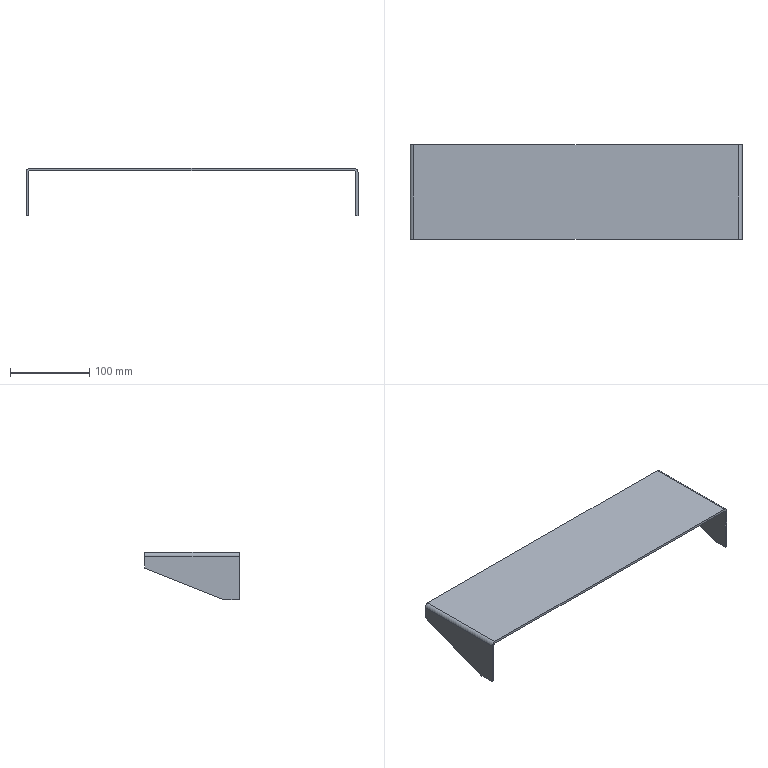Part | STEP file | HL4GZ-1.581.103 (tank support seat) | 1 solid | 16 faces | box 420 x 120 x 60 mm | volume 179158 mm3 | plane 12 | cylinder 4 | commonest cylinder face diameters 4 x2 10 x2
STEP:
#1=CARTESIAN_POINT('',(0.,0.,0.));
#2=DIRECTION('',(0.,0.,1.));
#3=DIRECTION('',(1.,0.,0.));
#4=AXIS2_PLACEMENT_3D('',#1,#2,#3);
#5=CARTESIAN_POINT('',(1598.,-510.,-385.));
#6=VERTEX_POINT('',#5);
#7=CARTESIAN_POINT('',(1598.,-410.,-345.));
#8=VERTEX_POINT('',#7);
#9=CARTESIAN_POINT('',(1598.,-420.345,-349.138));
#10=DIRECTION('',(0.,0.9285,0.3714));
#11=VECTOR('',#10,1.);
#12=LINE('',#9,#11);
#13=CARTESIAN_POINT('',(1956.277,-410.,-345.));
#14=DIRECTION('',(0.,-0.3714,0.9285));
#15=DIRECTION('',(1.,0.,0.));
#16=AXIS2_PLACEMENT_3D('',#13,#14,#15);
#17=PLANE('',#16);
#18=CARTESIAN_POINT('',(-358.277,-11.142));
#19=DIRECTION('',(0.,1.));
#20=VECTOR('',#19,1.);
#21=LINE('',#18,#20);
#22=(GEOMETRIC_REPRESENTATION_CONTEXT(2)PARAMETRIC_REPRESENTATION_CONTEXT()REPRESENTATION_CONTEXT('',''));
#23=DEFINITIONAL_REPRESENTATION('',(#21),#22);
#24=PCURVE('',#17,#23);
#25=CARTESIAN_POINT('',(1598.,-430.,-325.));
#26=DIRECTION('',(1.,0.,0.));
#27=DIRECTION('',(0.,0.,1.));
#28=AXIS2_PLACEMENT_3D('',#25,#26,#27);
#29=PLANE('',#28);
#30=CARTESIAN_POINT('',(-24.138,-9.655));
#31=DIRECTION('',(0.3714,-0.9285));
#32=VECTOR('',#31,1.);
#33=LINE('',#30,#32);
#34=(GEOMETRIC_REPRESENTATION_CONTEXT(2)PARAMETRIC_REPRESENTATION_CONTEXT()REPRESENTATION_CONTEXT('',''));
#35=DEFINITIONAL_REPRESENTATION('',(#33),#34);
#36=PCURVE('',#29,#35);
#37=SURFACE_CURVE('',#12,(#24,#36),.PCURVE_S1.);
#38=EDGE_CURVE('',#6,#8,#37,.T.);
#39=ORIENTED_EDGE('',*,*,#38,.F.);
#40=CARTESIAN_POINT('',(1595.,-510.,-385.));
#41=VERTEX_POINT('',#40);
#42=CARTESIAN_POINT('',(1595.,-510.,-385.));
#43=DIRECTION('',(1.,0.,0.));
#44=VECTOR('',#43,1.);
#45=LINE('',#42,#44);
#46=CARTESIAN_POINT('',(-361.277,-107.703));
#47=DIRECTION('',(1.,0.));
#48=VECTOR('',#47,1.);
#49=LINE('',#46,#48);
#50=(GEOMETRIC_REPRESENTATION_CONTEXT(2)PARAMETRIC_REPRESENTATION_CONTEXT()REPRESENTATION_CONTEXT('',''));
#51=DEFINITIONAL_REPRESENTATION('',(#49),#50);
#52=PCURVE('',#17,#51);
#53=CARTESIAN_POINT('',(1595.,-430.,-385.));
#54=DIRECTION('',(0.,0.,1.));
#55=DIRECTION('',(0.,1.,0.));
#56=AXIS2_PLACEMENT_3D('',#53,#54,#55);
#57=PLANE('',#56);
#58=CARTESIAN_POINT('',(-80.,0.));
#59=DIRECTION('',(0.,-1.));
#60=VECTOR('',#59,1.);
#61=LINE('',#58,#60);
#62=(GEOMETRIC_REPRESENTATION_CONTEXT(2)PARAMETRIC_REPRESENTATION_CONTEXT()REPRESENTATION_CONTEXT('',''));
#63=DEFINITIONAL_REPRESENTATION('',(#61),#62);
#64=PCURVE('',#57,#63);
#65=SURFACE_CURVE('',#45,(#52,#64),.PCURVE_S1.);
#66=EDGE_CURVE('',#41,#6,#65,.T.);
#67=ORIENTED_EDGE('',*,*,#66,.F.);
#68=CARTESIAN_POINT('',(1595.,-410.,-345.));
#69=VERTEX_POINT('',#68);
#70=CARTESIAN_POINT('',(1595.,-403.103,-342.241));
#71=DIRECTION('',(0.,-0.9285,-0.3714));
#72=VECTOR('',#71,1.);
#73=LINE('',#70,#72);
#74=CARTESIAN_POINT('',(-361.277,7.428));
#75=DIRECTION('',(0.,-1.));
#76=VECTOR('',#75,1.);
#77=LINE('',#74,#76);
#78=(GEOMETRIC_REPRESENTATION_CONTEXT(2)PARAMETRIC_REPRESENTATION_CONTEXT()REPRESENTATION_CONTEXT('',''));
#79=DEFINITIONAL_REPRESENTATION('',(#77),#78);
#80=PCURVE('',#17,#79);
#81=CARTESIAN_POINT('',(1595.,-410.,-325.));
#82=DIRECTION('',(1.,0.,0.));
#83=DIRECTION('',(0.,1.,0.));
#84=AXIS2_PLACEMENT_3D('',#81,#82,#83);
#85=PLANE('',#84);
#86=CARTESIAN_POINT('',(6.897,-17.241));
#87=DIRECTION('',(-0.9285,-0.3714));
#88=VECTOR('',#87,1.);
#89=LINE('',#86,#88);
#90=(GEOMETRIC_REPRESENTATION_CONTEXT(2)PARAMETRIC_REPRESENTATION_CONTEXT()REPRESENTATION_CONTEXT('',''));
#91=DEFINITIONAL_REPRESENTATION('',(#89),#90);
#92=PCURVE('',#85,#91);
#93=SURFACE_CURVE('',#73,(#80,#92),.PCURVE_S1.);
#94=EDGE_CURVE('',#69,#41,#93,.T.);
#95=ORIENTED_EDGE('',*,*,#94,.F.);
#96=CARTESIAN_POINT('',(1956.277,-410.,-345.));
#97=DIRECTION('',(-1.,0.,0.));
#98=VECTOR('',#97,1.);
#99=LINE('',#96,#98);
#100=CARTESIAN_POINT('',(0.,0.));
#101=DIRECTION('',(-1.,0.));
#102=VECTOR('',#101,1.);
#103=LINE('',#100,#102);
#104=(GEOMETRIC_REPRESENTATION_CONTEXT(2)PARAMETRIC_REPRESENTATION_CONTEXT()REPRESENTATION_CONTEXT('',''));
#105=DEFINITIONAL_REPRESENTATION('',(#103),#104);
#106=PCURVE('',#17,#105);
#107=CARTESIAN_POINT('',(1956.277,-410.,-325.));
#108=DIRECTION('',(0.,-1.,0.));
#109=DIRECTION('',(1.,0.,0.));
#110=AXIS2_PLACEMENT_3D('',#107,#108,#109);
#111=PLANE('',#110);
#112=CARTESIAN_POINT('',(0.,-20.));
#113=DIRECTION('',(-1.,0.));
#114=VECTOR('',#113,1.);
#115=LINE('',#112,#114);
#116=(GEOMETRIC_REPRESENTATION_CONTEXT(2)PARAMETRIC_REPRESENTATION_CONTEXT()REPRESENTATION_CONTEXT('',''));
#117=DEFINITIONAL_REPRESENTATION('',(#115),#116);
#118=PCURVE('',#111,#117);
#119=SURFACE_CURVE('',#99,(#106,#118),.PCURVE_S1.);
#120=EDGE_CURVE('',#8,#69,#119,.T.);
#121=ORIENTED_EDGE('',*,*,#120,.F.);
#122=EDGE_LOOP('',(#39,#67,#95,#121));
#123=FACE_BOUND('',#122,.T.);
#124=ADVANCED_FACE('',(#123),#17,.F.);
#125=CARTESIAN_POINT('',(2015.,-510.,-385.));
#126=VERTEX_POINT('',#125);
#127=CARTESIAN_POINT('',(2015.,-410.,-345.));
#128=VERTEX_POINT('',#127);
#129=CARTESIAN_POINT('',(2015.,-612.586,-426.034));
#130=DIRECTION('',(0.,0.9285,0.3714));
#131=VECTOR('',#130,1.);
#132=LINE('',#129,#131);
#133=CARTESIAN_POINT('',(1956.277,-410.,-345.));
#134=DIRECTION('',(0.,-0.3714,0.9285));
#135=DIRECTION('',(1.,0.,0.));
#136=AXIS2_PLACEMENT_3D('',#133,#134,#135);
#137=PLANE('',#136);
#138=CARTESIAN_POINT('',(58.723,-218.192));
#139=DIRECTION('',(0.,1.));
#140=VECTOR('',#139,1.);
#141=LINE('',#138,#140);
#142=(GEOMETRIC_REPRESENTATION_CONTEXT(2)PARAMETRIC_REPRESENTATION_CONTEXT()REPRESENTATION_CONTEXT('',''));
#143=DEFINITIONAL_REPRESENTATION('',(#141),#142);
#144=PCURVE('',#137,#143);
#145=CARTESIAN_POINT('',(2015.,-653.,-325.));
#146=DIRECTION('',(1.,0.,0.));
#147=DIRECTION('',(0.,1.,0.));
#148=AXIS2_PLACEMENT_3D('',#145,#146,#147);
#149=PLANE('',#148);
#150=CARTESIAN_POINT('',(40.414,-101.034));
#151=DIRECTION('',(0.9285,0.3714));
#152=VECTOR('',#151,1.);
#153=LINE('',#150,#152);
#154=(GEOMETRIC_REPRESENTATION_CONTEXT(2)PARAMETRIC_REPRESENTATION_CONTEXT()REPRESENTATION_CONTEXT('',''));
#155=DEFINITIONAL_REPRESENTATION('',(#153),#154);
#156=PCURVE('',#149,#155);
#157=SURFACE_CURVE('',#132,(#144,#156),.PCURVE_S1.);
#158=EDGE_CURVE('',#126,#128,#157,.T.);
#159=ORIENTED_EDGE('',*,*,#158,.F.);
#160=CARTESIAN_POINT('',(2012.,-510.,-385.));
#161=VERTEX_POINT('',#160);
#162=CARTESIAN_POINT('',(2015.,-510.,-385.));
#163=DIRECTION('',(1.,0.,0.));
#164=VECTOR('',#163,1.);
#165=LINE('',#162,#164);
#166=CARTESIAN_POINT('',(58.723,-107.703));
#167=DIRECTION('',(1.,0.));
#168=VECTOR('',#167,1.);
#169=LINE('',#166,#168);
#170=(GEOMETRIC_REPRESENTATION_CONTEXT(2)PARAMETRIC_REPRESENTATION_CONTEXT()REPRESENTATION_CONTEXT('',''));
#171=DEFINITIONAL_REPRESENTATION('',(#169),#170);
#172=PCURVE('',#137,#171);
#173=CARTESIAN_POINT('',(2015.,-430.,-385.));
#174=DIRECTION('',(0.,0.,1.));
#175=DIRECTION('',(0.,1.,0.));
#176=AXIS2_PLACEMENT_3D('',#173,#174,#175);
#177=PLANE('',#176);
#178=CARTESIAN_POINT('',(-80.,0.));
#179=DIRECTION('',(0.,-1.));
#180=VECTOR('',#179,1.);
#181=LINE('',#178,#180);
#182=(GEOMETRIC_REPRESENTATION_CONTEXT(2)PARAMETRIC_REPRESENTATION_CONTEXT()REPRESENTATION_CONTEXT('',''));
#183=DEFINITIONAL_REPRESENTATION('',(#181),#182);
#184=PCURVE('',#177,#183);
#185=SURFACE_CURVE('',#165,(#172,#184),.PCURVE_S1.);
#186=EDGE_CURVE('',#161,#126,#185,.T.);
#187=ORIENTED_EDGE('',*,*,#186,.F.);
#188=CARTESIAN_POINT('',(2012.,-410.,-345.));
#189=VERTEX_POINT('',#188);
#190=CARTESIAN_POINT('',(2012.,-420.345,-349.138));
#191=DIRECTION('',(0.,-0.9285,-0.3714));
#192=VECTOR('',#191,1.);
#193=LINE('',#190,#192);
#194=CARTESIAN_POINT('',(55.723,-11.142));
#195=DIRECTION('',(0.,-1.));
#196=VECTOR('',#195,1.);
#197=LINE('',#194,#196);
#198=(GEOMETRIC_REPRESENTATION_CONTEXT(2)PARAMETRIC_REPRESENTATION_CONTEXT()REPRESENTATION_CONTEXT('',''));
#199=DEFINITIONAL_REPRESENTATION('',(#197),#198);
#200=PCURVE('',#137,#199);
#201=CARTESIAN_POINT('',(2012.,-430.,-325.));
#202=DIRECTION('',(-1.,0.,0.));
#203=DIRECTION('',(0.,0.,1.));
#204=AXIS2_PLACEMENT_3D('',#201,#202,#203);
#205=PLANE('',#204);
#206=CARTESIAN_POINT('',(-24.138,9.655));
#207=DIRECTION('',(-0.3714,-0.9285));
#208=VECTOR('',#207,1.);
#209=LINE('',#206,#208);
#210=(GEOMETRIC_REPRESENTATION_CONTEXT(2)PARAMETRIC_REPRESENTATION_CONTEXT()REPRESENTATION_CONTEXT('',''));
#211=DEFINITIONAL_REPRESENTATION('',(#209),#210);
#212=PCURVE('',#205,#211);
#213=SURFACE_CURVE('',#193,(#200,#212),.PCURVE_S1.);
#214=EDGE_CURVE('',#189,#161,#213,.T.);
#215=ORIENTED_EDGE('',*,*,#214,.F.);
#216=CARTESIAN_POINT('',(1956.277,-410.,-345.));
#217=DIRECTION('',(-1.,0.,0.));
#218=VECTOR('',#217,1.);
#219=LINE('',#216,#218);
#220=CARTESIAN_POINT('',(0.,0.));
#221=DIRECTION('',(-1.,0.));
#222=VECTOR('',#221,1.);
#223=LINE('',#220,#222);
#224=(GEOMETRIC_REPRESENTATION_CONTEXT(2)PARAMETRIC_REPRESENTATION_CONTEXT()REPRESENTATION_CONTEXT('',''));
#225=DEFINITIONAL_REPRESENTATION('',(#223),#224);
#226=PCURVE('',#137,#225);
#227=CARTESIAN_POINT('',(0.,-20.));
#228=DIRECTION('',(-1.,0.));
#229=VECTOR('',#228,1.);
#230=LINE('',#227,#229);
#231=(GEOMETRIC_REPRESENTATION_CONTEXT(2)PARAMETRIC_REPRESENTATION_CONTEXT()REPRESENTATION_CONTEXT('',''));
#232=DEFINITIONAL_REPRESENTATION('',(#230),#231);
#233=PCURVE('',#111,#232);
#234=SURFACE_CURVE('',#219,(#226,#233),.PCURVE_S1.);
#235=EDGE_CURVE('',#128,#189,#234,.T.);
#236=ORIENTED_EDGE('',*,*,#235,.F.);
#237=EDGE_LOOP('',(#159,#187,#215,#236));
#238=FACE_BOUND('',#237,.T.);
#239=ADVANCED_FACE('',(#238),#137,.F.);
#240=CARTESIAN_POINT('',(2010.,-410.,-325.));
#241=VERTEX_POINT('',#240);
#242=CARTESIAN_POINT('',(2015.,-410.,-330.));
#243=VERTEX_POINT('',#242);
#244=CARTESIAN_POINT('',(2010.,-410.,-330.));
#245=DIRECTION('',(0.,1.,0.));
#246=DIRECTION('',(0.,0.,-1.));
#247=AXIS2_PLACEMENT_3D('',#244,#245,#246);
#248=CIRCLE('',#247,5.);
#249=CARTESIAN_POINT('',(2010.,-641.723,-330.));
#250=DIRECTION('',(0.,-1.,0.));
#251=DIRECTION('',(-1.,0.,0.));
#252=AXIS2_PLACEMENT_3D('',#249,#250,#251);
#253=CYLINDRICAL_SURFACE('',#252,5.);
#254=CARTESIAN_POINT('',(7.854,-231.723));
#255=DIRECTION('',(-1.,0.));
#256=VECTOR('',#255,1.);
#257=LINE('',#254,#256);
#258=(GEOMETRIC_REPRESENTATION_CONTEXT(2)PARAMETRIC_REPRESENTATION_CONTEXT()REPRESENTATION_CONTEXT('',''));
#259=DEFINITIONAL_REPRESENTATION('',(#257),#258);
#260=PCURVE('',#253,#259);
#261=CARTESIAN_POINT('',(53.723,-10.));
#262=CARTESIAN_POINT('',(45.063,-10.));
#263=CARTESIAN_POINT('',(49.393,-2.5));
#264=CARTESIAN_POINT('',(53.723,5.));
#265=CARTESIAN_POINT('',(58.054,-2.5));
#266=CARTESIAN_POINT('',(62.384,-10.));
#267=CARTESIAN_POINT('',(53.723,-10.));
#268=(BOUNDED_CURVE()B_SPLINE_CURVE(2,(#261,#262,#263,#264,#265,#266,#267),.UNSPECIFIED.,.T.,.F.)B_SPLINE_CURVE_WITH_KNOTS((1,2,2,2,2,1),(-2.094,0.,2.094,4.189,6.283,8.378),.UNSPECIFIED.)CURVE()GEOMETRIC_REPRESENTATION_ITEM()RATIONAL_B_SPLINE_CURVE((1.,0.5,1.,0.5,1.,0.5,1.))REPRESENTATION_ITEM(''));
#269=(GEOMETRIC_REPRESENTATION_CONTEXT(2)PARAMETRIC_REPRESENTATION_CONTEXT()REPRESENTATION_CONTEXT('',''));
#270=DEFINITIONAL_REPRESENTATION('',(#268),#269);
#271=PCURVE('',#111,#270);
#272=SURFACE_CURVE('',#248,(#260,#271),.PCURVE_S1.);
#273=EDGE_CURVE('',#241,#243,#272,.T.);
#274=ORIENTED_EDGE('',*,*,#273,.F.);
#275=CARTESIAN_POINT('',(2010.,-530.,-325.));
#276=VERTEX_POINT('',#275);
#277=CARTESIAN_POINT('',(2010.,-641.723,-325.));
#278=DIRECTION('',(0.,1.,0.));
#279=VECTOR('',#278,1.);
#280=LINE('',#277,#279);
#281=CARTESIAN_POINT('',(4.712,0.));
#282=DIRECTION('',(0.,-1.));
#283=VECTOR('',#282,1.);
#284=LINE('',#281,#283);
#285=(GEOMETRIC_REPRESENTATION_CONTEXT(2)PARAMETRIC_REPRESENTATION_CONTEXT()REPRESENTATION_CONTEXT('',''));
#286=DEFINITIONAL_REPRESENTATION('',(#284),#285);
#287=PCURVE('',#253,#286);
#288=CARTESIAN_POINT('',(1956.277,-641.723,-325.));
#289=DIRECTION('',(0.,0.,-1.));
#290=DIRECTION('',(1.,0.,0.));
#291=AXIS2_PLACEMENT_3D('',#288,#289,#290);
#292=PLANE('',#291);
#293=CARTESIAN_POINT('',(53.723,0.));
#294=DIRECTION('',(0.,-1.));
#295=VECTOR('',#294,1.);
#296=LINE('',#293,#295);
#297=(GEOMETRIC_REPRESENTATION_CONTEXT(2)PARAMETRIC_REPRESENTATION_CONTEXT()REPRESENTATION_CONTEXT('',''));
#298=DEFINITIONAL_REPRESENTATION('',(#296),#297);
#299=PCURVE('',#292,#298);
#300=SURFACE_CURVE('',#280,(#287,#299),.PCURVE_S1.);
#301=EDGE_CURVE('',#276,#241,#300,.T.);
#302=ORIENTED_EDGE('',*,*,#301,.F.);
#303=CARTESIAN_POINT('',(2015.,-530.,-330.));
#304=VERTEX_POINT('',#303);
#305=CARTESIAN_POINT('',(2010.,-530.,-330.));
#306=DIRECTION('',(0.,-1.,0.));
#307=DIRECTION('',(0.,0.,-1.));
#308=AXIS2_PLACEMENT_3D('',#305,#306,#307);
#309=CIRCLE('',#308,5.);
#310=CARTESIAN_POINT('',(1.571,-111.723));
#311=DIRECTION('',(1.,0.));
#312=VECTOR('',#311,1.);
#313=LINE('',#310,#312);
#314=(GEOMETRIC_REPRESENTATION_CONTEXT(2)PARAMETRIC_REPRESENTATION_CONTEXT()REPRESENTATION_CONTEXT('',''));
#315=DEFINITIONAL_REPRESENTATION('',(#313),#314);
#316=PCURVE('',#253,#315);
#317=CARTESIAN_POINT('',(1855.,-530.,-355.));
#318=DIRECTION('',(0.,-1.,0.));
#319=DIRECTION('',(0.,0.,1.));
#320=AXIS2_PLACEMENT_3D('',#317,#318,#319);
#321=PLANE('',#320);
#322=CARTESIAN_POINT('',(25.,-155.));
#323=DIRECTION('',(-1.,0.));
#324=AXIS2_PLACEMENT_2D('',#322,#323);
#325=CIRCLE('',#324,5.);
#326=(GEOMETRIC_REPRESENTATION_CONTEXT(2)PARAMETRIC_REPRESENTATION_CONTEXT()REPRESENTATION_CONTEXT('',''));
#327=DEFINITIONAL_REPRESENTATION('',(#325),#326);
#328=PCURVE('',#321,#327);
#329=SURFACE_CURVE('',#309,(#316,#328),.PCURVE_S1.);
#330=EDGE_CURVE('',#304,#276,#329,.T.);
#331=ORIENTED_EDGE('',*,*,#330,.F.);
#332=CARTESIAN_POINT('',(2015.,-641.723,-330.));
#333=DIRECTION('',(0.,-1.,0.));
#334=VECTOR('',#333,1.);
#335=LINE('',#332,#334);
#336=CARTESIAN_POINT('',(3.142,0.));
#337=DIRECTION('',(0.,1.));
#338=VECTOR('',#337,1.);
#339=LINE('',#336,#338);
#340=(GEOMETRIC_REPRESENTATION_CONTEXT(2)PARAMETRIC_REPRESENTATION_CONTEXT()REPRESENTATION_CONTEXT('',''));
#341=DEFINITIONAL_REPRESENTATION('',(#339),#340);
#342=PCURVE('',#253,#341);
#343=CARTESIAN_POINT('',(11.277,-5.));
#344=DIRECTION('',(-1.,0.));
#345=VECTOR('',#344,1.);
#346=LINE('',#343,#345);
#347=(GEOMETRIC_REPRESENTATION_CONTEXT(2)PARAMETRIC_REPRESENTATION_CONTEXT()REPRESENTATION_CONTEXT('',''));
#348=DEFINITIONAL_REPRESENTATION('',(#346),#347);
#349=PCURVE('',#149,#348);
#350=SURFACE_CURVE('',#335,(#342,#349),.PCURVE_S1.);
#351=EDGE_CURVE('',#243,#304,#350,.T.);
#352=ORIENTED_EDGE('',*,*,#351,.F.);
#353=EDGE_LOOP('',(#274,#302,#331,#352));
#354=FACE_BOUND('',#353,.T.);
#355=ADVANCED_FACE('',(#354),#253,.T.);
#356=CARTESIAN_POINT('',(1600.,-530.,-325.));
#357=VERTEX_POINT('',#356);
#358=CARTESIAN_POINT('',(1595.,-530.,-330.));
#359=VERTEX_POINT('',#358);
#360=CARTESIAN_POINT('',(1600.,-530.,-330.));
#361=DIRECTION('',(0.,-1.,0.));
#362=DIRECTION('',(0.,0.,-1.));
#363=AXIS2_PLACEMENT_3D('',#360,#361,#362);
#364=CIRCLE('',#363,5.);
#365=CARTESIAN_POINT('',(1600.,-641.723,-330.));
#366=DIRECTION('',(0.,-1.,0.));
#367=DIRECTION('',(0.,0.,1.));
#368=AXIS2_PLACEMENT_3D('',#365,#366,#367);
#369=CYLINDRICAL_SURFACE('',#368,5.);
#370=CARTESIAN_POINT('',(-3.142,-111.723));
#371=DIRECTION('',(1.,0.));
#372=VECTOR('',#371,1.);
#373=LINE('',#370,#372);
#374=(GEOMETRIC_REPRESENTATION_CONTEXT(2)PARAMETRIC_REPRESENTATION_CONTEXT()REPRESENTATION_CONTEXT('',''));
#375=DEFINITIONAL_REPRESENTATION('',(#373),#374);
#376=PCURVE('',#369,#375);
#377=CARTESIAN_POINT('',(25.,255.));
#378=DIRECTION('',(-1.,0.));
#379=AXIS2_PLACEMENT_2D('',#377,#378);
#380=CIRCLE('',#379,5.);
#381=(GEOMETRIC_REPRESENTATION_CONTEXT(2)PARAMETRIC_REPRESENTATION_CONTEXT()REPRESENTATION_CONTEXT('',''));
#382=DEFINITIONAL_REPRESENTATION('',(#380),#381);
#383=PCURVE('',#321,#382);
#384=SURFACE_CURVE('',#364,(#376,#383),.PCURVE_S1.);
#385=EDGE_CURVE('',#357,#359,#384,.T.);
#386=ORIENTED_EDGE('',*,*,#385,.F.);
#387=CARTESIAN_POINT('',(1600.,-410.,-325.));
#388=VERTEX_POINT('',#387);
#389=CARTESIAN_POINT('',(1600.,-641.723,-325.));
#390=DIRECTION('',(0.,-1.,0.));
#391=VECTOR('',#390,1.);
#392=LINE('',#389,#391);
#393=CARTESIAN_POINT('',(0.,0.));
#394=DIRECTION('',(0.,1.));
#395=VECTOR('',#394,1.);
#396=LINE('',#393,#395);
#397=(GEOMETRIC_REPRESENTATION_CONTEXT(2)PARAMETRIC_REPRESENTATION_CONTEXT()REPRESENTATION_CONTEXT('',''));
#398=DEFINITIONAL_REPRESENTATION('',(#396),#397);
#399=PCURVE('',#369,#398);
#400=CARTESIAN_POINT('',(-356.277,0.));
#401=DIRECTION('',(0.,1.));
#402=VECTOR('',#401,1.);
#403=LINE('',#400,#402);
#404=(GEOMETRIC_REPRESENTATION_CONTEXT(2)PARAMETRIC_REPRESENTATION_CONTEXT()REPRESENTATION_CONTEXT('',''));
#405=DEFINITIONAL_REPRESENTATION('',(#403),#404);
#406=PCURVE('',#292,#405);
#407=SURFACE_CURVE('',#392,(#399,#406),.PCURVE_S1.);
#408=EDGE_CURVE('',#388,#357,#407,.T.);
#409=ORIENTED_EDGE('',*,*,#408,.F.);
#410=CARTESIAN_POINT('',(1595.,-410.,-330.));
#411=VERTEX_POINT('',#410);
#412=CARTESIAN_POINT('',(1600.,-410.,-330.));
#413=DIRECTION('',(0.,1.,0.));
#414=DIRECTION('',(0.,0.,-1.));
#415=AXIS2_PLACEMENT_3D('',#412,#413,#414);
#416=CIRCLE('',#415,5.);
#417=CARTESIAN_POINT('',(3.142,-231.723));
#418=DIRECTION('',(-1.,0.));
#419=VECTOR('',#418,1.);
#420=LINE('',#417,#419);
#421=(GEOMETRIC_REPRESENTATION_CONTEXT(2)PARAMETRIC_REPRESENTATION_CONTEXT()REPRESENTATION_CONTEXT('',''));
#422=DEFINITIONAL_REPRESENTATION('',(#420),#421);
#423=PCURVE('',#369,#422);
#424=CARTESIAN_POINT('',(-356.277,-10.));
#425=CARTESIAN_POINT('',(-364.937,-10.));
#426=CARTESIAN_POINT('',(-360.607,-2.5));
#427=CARTESIAN_POINT('',(-356.277,5.));
#428=CARTESIAN_POINT('',(-351.946,-2.5));
#429=CARTESIAN_POINT('',(-347.616,-10.));
#430=CARTESIAN_POINT('',(-356.277,-10.));
#431=(BOUNDED_CURVE()B_SPLINE_CURVE(2,(#424,#425,#426,#427,#428,#429,#430),.UNSPECIFIED.,.T.,.F.)B_SPLINE_CURVE_WITH_KNOTS((1,2,2,2,2,1),(-2.094,0.,2.094,4.189,6.283,8.378),.UNSPECIFIED.)CURVE()GEOMETRIC_REPRESENTATION_ITEM()RATIONAL_B_SPLINE_CURVE((1.,0.5,1.,0.5,1.,0.5,1.))REPRESENTATION_ITEM(''));
#432=(GEOMETRIC_REPRESENTATION_CONTEXT(2)PARAMETRIC_REPRESENTATION_CONTEXT()REPRESENTATION_CONTEXT('',''));
#433=DEFINITIONAL_REPRESENTATION('',(#431),#432);
#434=PCURVE('',#111,#433);
#435=SURFACE_CURVE('',#416,(#423,#434),.PCURVE_S1.);
#436=EDGE_CURVE('',#411,#388,#435,.T.);
#437=ORIENTED_EDGE('',*,*,#436,.F.);
#438=CARTESIAN_POINT('',(1595.,-641.723,-330.));
#439=DIRECTION('',(0.,1.,0.));
#440=VECTOR('',#439,1.);
#441=LINE('',#438,#440);
#442=CARTESIAN_POINT('',(1.571,0.));
#443=DIRECTION('',(0.,-1.));
#444=VECTOR('',#443,1.);
#445=LINE('',#442,#444);
#446=(GEOMETRIC_REPRESENTATION_CONTEXT(2)PARAMETRIC_REPRESENTATION_CONTEXT()REPRESENTATION_CONTEXT('',''));
#447=DEFINITIONAL_REPRESENTATION('',(#445),#446);
#448=PCURVE('',#369,#447);
#449=CARTESIAN_POINT('',(-231.723,-5.));
#450=DIRECTION('',(1.,0.));
#451=VECTOR('',#450,1.);
#452=LINE('',#449,#451);
#453=(GEOMETRIC_REPRESENTATION_CONTEXT(2)PARAMETRIC_REPRESENTATION_CONTEXT()REPRESENTATION_CONTEXT('',''));
#454=DEFINITIONAL_REPRESENTATION('',(#452),#453);
#455=PCURVE('',#85,#454);
#456=SURFACE_CURVE('',#441,(#448,#455),.PCURVE_S1.);
#457=EDGE_CURVE('',#359,#411,#456,.T.);
#458=ORIENTED_EDGE('',*,*,#457,.F.);
#459=EDGE_LOOP('',(#386,#409,#437,#458));
#460=FACE_BOUND('',#459,.T.);
#461=ADVANCED_FACE('',(#460),#369,.T.);
#462=CARTESIAN_POINT('',(1598.,-410.,-330.));
#463=VERTEX_POINT('',#462);
#464=CARTESIAN_POINT('',(1598.,-530.,-330.));
#465=VERTEX_POINT('',#464);
#466=CARTESIAN_POINT('',(1598.,-641.723,-330.));
#467=DIRECTION('',(0.,-1.,0.));
#468=VECTOR('',#467,1.);
#469=LINE('',#466,#468);
#470=CARTESIAN_POINT('',(1600.,-641.723,-330.));
#471=DIRECTION('',(0.,-1.,0.));
#472=DIRECTION('',(0.,0.,1.));
#473=AXIS2_PLACEMENT_3D('',#470,#471,#472);
#474=CYLINDRICAL_SURFACE('',#473,2.);
#475=CARTESIAN_POINT('',(1.571,0.));
#476=DIRECTION('',(0.,1.));
#477=VECTOR('',#476,1.);
#478=LINE('',#475,#477);
#479=(GEOMETRIC_REPRESENTATION_CONTEXT(2)PARAMETRIC_REPRESENTATION_CONTEXT()REPRESENTATION_CONTEXT('',''));
#480=DEFINITIONAL_REPRESENTATION('',(#478),#479);
#481=PCURVE('',#474,#480);
#482=CARTESIAN_POINT('',(-5.,211.723));
#483=DIRECTION('',(0.,1.));
#484=VECTOR('',#483,1.);
#485=LINE('',#482,#484);
#486=(GEOMETRIC_REPRESENTATION_CONTEXT(2)PARAMETRIC_REPRESENTATION_CONTEXT()REPRESENTATION_CONTEXT('',''));
#487=DEFINITIONAL_REPRESENTATION('',(#485),#486);
#488=PCURVE('',#29,#487);
#489=SURFACE_CURVE('',#469,(#481,#488),.PCURVE_S1.);
#490=EDGE_CURVE('',#463,#465,#489,.T.);
#491=ORIENTED_EDGE('',*,*,#490,.T.);
#492=CARTESIAN_POINT('',(1600.,-530.,-328.));
#493=VERTEX_POINT('',#492);
#494=CARTESIAN_POINT('',(1600.,-530.,-330.));
#495=DIRECTION('',(0.,1.,0.));
#496=DIRECTION('',(0.,0.,-1.));
#497=AXIS2_PLACEMENT_3D('',#494,#495,#496);
#498=CIRCLE('',#497,2.);
#499=CARTESIAN_POINT('',(3.142,-111.723));
#500=DIRECTION('',(-1.,0.));
#501=VECTOR('',#500,1.);
#502=LINE('',#499,#501);
#503=(GEOMETRIC_REPRESENTATION_CONTEXT(2)PARAMETRIC_REPRESENTATION_CONTEXT()REPRESENTATION_CONTEXT('',''));
#504=DEFINITIONAL_REPRESENTATION('',(#502),#503);
#505=PCURVE('',#474,#504);
#506=CARTESIAN_POINT('',(23.,255.));
#507=CARTESIAN_POINT('',(23.,258.464));
#508=CARTESIAN_POINT('',(26.,256.732));
#509=CARTESIAN_POINT('',(29.,255.));
#510=CARTESIAN_POINT('',(26.,253.268));
#511=CARTESIAN_POINT('',(23.,251.536));
#512=CARTESIAN_POINT('',(23.,255.));
#513=(BOUNDED_CURVE()B_SPLINE_CURVE(2,(#506,#507,#508,#509,#510,#511,#512),.UNSPECIFIED.,.T.,.F.)B_SPLINE_CURVE_WITH_KNOTS((1,2,2,2,2,1),(-2.094,0.,2.094,4.189,6.283,8.378),.UNSPECIFIED.)CURVE()GEOMETRIC_REPRESENTATION_ITEM()RATIONAL_B_SPLINE_CURVE((1.,0.5,1.,0.5,1.,0.5,1.))REPRESENTATION_ITEM(''));
#514=(GEOMETRIC_REPRESENTATION_CONTEXT(2)PARAMETRIC_REPRESENTATION_CONTEXT()REPRESENTATION_CONTEXT('',''));
#515=DEFINITIONAL_REPRESENTATION('',(#513),#514);
#516=PCURVE('',#321,#515);
#517=SURFACE_CURVE('',#498,(#505,#516),.PCURVE_S1.);
#518=EDGE_CURVE('',#465,#493,#517,.T.);
#519=ORIENTED_EDGE('',*,*,#518,.T.);
#520=CARTESIAN_POINT('',(1600.,-410.,-328.));
#521=VERTEX_POINT('',#520);
#522=CARTESIAN_POINT('',(1600.,-641.723,-328.));
#523=DIRECTION('',(0.,1.,0.));
#524=VECTOR('',#523,1.);
#525=LINE('',#522,#524);
#526=CARTESIAN_POINT('',(0.,0.));
#527=DIRECTION('',(0.,-1.));
#528=VECTOR('',#527,1.);
#529=LINE('',#526,#528);
#530=(GEOMETRIC_REPRESENTATION_CONTEXT(2)PARAMETRIC_REPRESENTATION_CONTEXT()REPRESENTATION_CONTEXT('',''));
#531=DEFINITIONAL_REPRESENTATION('',(#529),#530);
#532=PCURVE('',#474,#531);
#533=CARTESIAN_POINT('',(1956.277,-641.723,-328.));
#534=DIRECTION('',(0.,0.,-1.));
#535=DIRECTION('',(1.,0.,0.));
#536=AXIS2_PLACEMENT_3D('',#533,#534,#535);
#537=PLANE('',#536);
#538=CARTESIAN_POINT('',(-356.277,0.));
#539=DIRECTION('',(0.,-1.));
#540=VECTOR('',#539,1.);
#541=LINE('',#538,#540);
#542=(GEOMETRIC_REPRESENTATION_CONTEXT(2)PARAMETRIC_REPRESENTATION_CONTEXT()REPRESENTATION_CONTEXT('',''));
#543=DEFINITIONAL_REPRESENTATION('',(#541),#542);
#544=PCURVE('',#537,#543);
#545=SURFACE_CURVE('',#525,(#532,#544),.PCURVE_S1.);
#546=EDGE_CURVE('',#493,#521,#545,.T.);
#547=ORIENTED_EDGE('',*,*,#546,.T.);
#548=CARTESIAN_POINT('',(1600.,-410.,-330.));
#549=DIRECTION('',(0.,-1.,0.));
#550=DIRECTION('',(0.,0.,-1.));
#551=AXIS2_PLACEMENT_3D('',#548,#549,#550);
#552=CIRCLE('',#551,2.);
#553=CARTESIAN_POINT('',(-3.142,-231.723));
#554=DIRECTION('',(1.,0.));
#555=VECTOR('',#554,1.);
#556=LINE('',#553,#555);
#557=(GEOMETRIC_REPRESENTATION_CONTEXT(2)PARAMETRIC_REPRESENTATION_CONTEXT()REPRESENTATION_CONTEXT('',''));
#558=DEFINITIONAL_REPRESENTATION('',(#556),#557);
#559=PCURVE('',#474,#558);
#560=CARTESIAN_POINT('',(-356.277,-5.));
#561=DIRECTION('',(0.,-1.));
#562=AXIS2_PLACEMENT_2D('',#560,#561);
#563=CIRCLE('',#562,2.);
#564=(GEOMETRIC_REPRESENTATION_CONTEXT(2)PARAMETRIC_REPRESENTATION_CONTEXT()REPRESENTATION_CONTEXT('',''));
#565=DEFINITIONAL_REPRESENTATION('',(#563),#564);
#566=PCURVE('',#111,#565);
#567=SURFACE_CURVE('',#552,(#559,#566),.PCURVE_S1.);
#568=EDGE_CURVE('',#521,#463,#567,.T.);
#569=ORIENTED_EDGE('',*,*,#568,.T.);
#570=EDGE_LOOP('',(#491,#519,#547,#569));
#571=FACE_BOUND('',#570,.F.);
#572=ADVANCED_FACE('',(#571),#474,.F.);
#573=CARTESIAN_POINT('',(2012.,-530.,-330.));
#574=VERTEX_POINT('',#573);
#575=CARTESIAN_POINT('',(2012.,-410.,-330.));
#576=VERTEX_POINT('',#575);
#577=CARTESIAN_POINT('',(2012.,-641.723,-330.));
#578=DIRECTION('',(0.,1.,0.));
#579=VECTOR('',#578,1.);
#580=LINE('',#577,#579);
#581=CARTESIAN_POINT('',(2010.,-641.723,-330.));
#582=DIRECTION('',(0.,1.,0.));
#583=DIRECTION('',(0.,0.,-1.));
#584=AXIS2_PLACEMENT_3D('',#581,#582,#583);
#585=CYLINDRICAL_SURFACE('',#584,2.);
#586=CARTESIAN_POINT('',(4.712,0.));
#587=DIRECTION('',(0.,1.));
#588=VECTOR('',#587,1.);
#589=LINE('',#586,#588);
#590=(GEOMETRIC_REPRESENTATION_CONTEXT(2)PARAMETRIC_REPRESENTATION_CONTEXT()REPRESENTATION_CONTEXT('',''));
#591=DEFINITIONAL_REPRESENTATION('',(#589),#590);
#592=PCURVE('',#585,#591);
#593=CARTESIAN_POINT('',(-5.,-211.723));
#594=DIRECTION('',(0.,1.));
#595=VECTOR('',#594,1.);
#596=LINE('',#593,#595);
#597=(GEOMETRIC_REPRESENTATION_CONTEXT(2)PARAMETRIC_REPRESENTATION_CONTEXT()REPRESENTATION_CONTEXT('',''));
#598=DEFINITIONAL_REPRESENTATION('',(#596),#597);
#599=PCURVE('',#205,#598);
#600=SURFACE_CURVE('',#580,(#592,#599),.PCURVE_S1.);
#601=EDGE_CURVE('',#574,#576,#600,.T.);
#602=ORIENTED_EDGE('',*,*,#601,.T.);
#603=CARTESIAN_POINT('',(2010.,-410.,-328.));
#604=VERTEX_POINT('',#603);
#605=CARTESIAN_POINT('',(2010.,-410.,-330.));
#606=DIRECTION('',(0.,-1.,0.));
#607=DIRECTION('',(0.,0.,-1.));
#608=AXIS2_PLACEMENT_3D('',#605,#606,#607);
#609=CIRCLE('',#608,2.);
#610=CARTESIAN_POINT('',(6.283,231.723));
#611=DIRECTION('',(-1.,0.));
#612=VECTOR('',#611,1.);
#613=LINE('',#610,#612);
#614=(GEOMETRIC_REPRESENTATION_CONTEXT(2)PARAMETRIC_REPRESENTATION_CONTEXT()REPRESENTATION_CONTEXT('',''));
#615=DEFINITIONAL_REPRESENTATION('',(#613),#614);
#616=PCURVE('',#585,#615);
#617=CARTESIAN_POINT('',(53.723,-5.));
#618=DIRECTION('',(0.,-1.));
#619=AXIS2_PLACEMENT_2D('',#617,#618);
#620=CIRCLE('',#619,2.);
#621=(GEOMETRIC_REPRESENTATION_CONTEXT(2)PARAMETRIC_REPRESENTATION_CONTEXT()REPRESENTATION_CONTEXT('',''));
#622=DEFINITIONAL_REPRESENTATION('',(#620),#621);
#623=PCURVE('',#111,#622);
#624=SURFACE_CURVE('',#609,(#616,#623),.PCURVE_S1.);
#625=EDGE_CURVE('',#576,#604,#624,.T.);
#626=ORIENTED_EDGE('',*,*,#625,.T.);
#627=CARTESIAN_POINT('',(2010.,-530.,-328.));
#628=VERTEX_POINT('',#627);
#629=CARTESIAN_POINT('',(2010.,-641.723,-328.));
#630=DIRECTION('',(0.,-1.,0.));
#631=VECTOR('',#630,1.);
#632=LINE('',#629,#631);
#633=CARTESIAN_POINT('',(3.142,0.));
#634=DIRECTION('',(0.,-1.));
#635=VECTOR('',#634,1.);
#636=LINE('',#633,#635);
#637=(GEOMETRIC_REPRESENTATION_CONTEXT(2)PARAMETRIC_REPRESENTATION_CONTEXT()REPRESENTATION_CONTEXT('',''));
#638=DEFINITIONAL_REPRESENTATION('',(#636),#637);
#639=PCURVE('',#585,#638);
#640=CARTESIAN_POINT('',(53.723,0.));
#641=DIRECTION('',(0.,1.));
#642=VECTOR('',#641,1.);
#643=LINE('',#640,#642);
#644=(GEOMETRIC_REPRESENTATION_CONTEXT(2)PARAMETRIC_REPRESENTATION_CONTEXT()REPRESENTATION_CONTEXT('',''));
#645=DEFINITIONAL_REPRESENTATION('',(#643),#644);
#646=PCURVE('',#537,#645);
#647=SURFACE_CURVE('',#632,(#639,#646),.PCURVE_S1.);
#648=EDGE_CURVE('',#604,#628,#647,.T.);
#649=ORIENTED_EDGE('',*,*,#648,.T.);
#650=CARTESIAN_POINT('',(2010.,-530.,-330.));
#651=DIRECTION('',(0.,1.,0.));
#652=DIRECTION('',(0.,0.,-1.));
#653=AXIS2_PLACEMENT_3D('',#650,#651,#652);
#654=CIRCLE('',#653,2.);
#655=CARTESIAN_POINT('',(0.,111.723));
#656=DIRECTION('',(1.,0.));
#657=VECTOR('',#656,1.);
#658=LINE('',#655,#657);
#659=(GEOMETRIC_REPRESENTATION_CONTEXT(2)PARAMETRIC_REPRESENTATION_CONTEXT()REPRESENTATION_CONTEXT('',''));
#660=DEFINITIONAL_REPRESENTATION('',(#658),#659);
#661=PCURVE('',#585,#660);
#662=CARTESIAN_POINT('',(23.,-155.));
#663=CARTESIAN_POINT('',(23.,-151.536));
#664=CARTESIAN_POINT('',(26.,-153.268));
#665=CARTESIAN_POINT('',(29.,-155.));
#666=CARTESIAN_POINT('',(26.,-156.732));
#667=CARTESIAN_POINT('',(23.,-158.464));
#668=CARTESIAN_POINT('',(23.,-155.));
#669=(BOUNDED_CURVE()B_SPLINE_CURVE(2,(#662,#663,#664,#665,#666,#667,#668),.UNSPECIFIED.,.T.,.F.)B_SPLINE_CURVE_WITH_KNOTS((1,2,2,2,2,1),(-2.094,0.,2.094,4.189,6.283,8.378),.UNSPECIFIED.)CURVE()GEOMETRIC_REPRESENTATION_ITEM()RATIONAL_B_SPLINE_CURVE((1.,0.5,1.,0.5,1.,0.5,1.))REPRESENTATION_ITEM(''));
#670=(GEOMETRIC_REPRESENTATION_CONTEXT(2)PARAMETRIC_REPRESENTATION_CONTEXT()REPRESENTATION_CONTEXT('',''));
#671=DEFINITIONAL_REPRESENTATION('',(#669),#670);
#672=PCURVE('',#321,#671);
#673=SURFACE_CURVE('',#654,(#661,#672),.PCURVE_S1.);
#674=EDGE_CURVE('',#628,#574,#673,.T.);
#675=ORIENTED_EDGE('',*,*,#674,.T.);
#676=EDGE_LOOP('',(#602,#626,#649,#675));
#677=FACE_BOUND('',#676,.F.);
#678=ADVANCED_FACE('',(#677),#585,.F.);
#679=CARTESIAN_POINT('',(2012.,-410.,-325.));
#680=DIRECTION('',(0.,0.,-1.));
#681=VECTOR('',#680,1.);
#682=LINE('',#679,#681);
#683=CARTESIAN_POINT('',(0.,20.));
#684=DIRECTION('',(-1.,0.));
#685=VECTOR('',#684,1.);
#686=LINE('',#683,#685);
#687=(GEOMETRIC_REPRESENTATION_CONTEXT(2)PARAMETRIC_REPRESENTATION_CONTEXT()REPRESENTATION_CONTEXT('',''));
#688=DEFINITIONAL_REPRESENTATION('',(#686),#687);
#689=PCURVE('',#205,#688);
#690=CARTESIAN_POINT('',(55.723,0.));
#691=DIRECTION('',(0.,-1.));
#692=VECTOR('',#691,1.);
#693=LINE('',#690,#692);
#694=(GEOMETRIC_REPRESENTATION_CONTEXT(2)PARAMETRIC_REPRESENTATION_CONTEXT()REPRESENTATION_CONTEXT('',''));
#695=DEFINITIONAL_REPRESENTATION('',(#693),#694);
#696=PCURVE('',#111,#695);
#697=SURFACE_CURVE('',#682,(#689,#696),.PCURVE_S1.);
#698=EDGE_CURVE('',#576,#189,#697,.T.);
#699=ORIENTED_EDGE('',*,*,#698,.T.);
#700=ORIENTED_EDGE('',*,*,#214,.T.);
#701=CARTESIAN_POINT('',(2012.,-530.,-385.));
#702=VERTEX_POINT('',#701);
#703=CARTESIAN_POINT('',(2012.,-430.,-385.));
#704=DIRECTION('',(0.,-1.,0.));
#705=VECTOR('',#704,1.);
#706=LINE('',#703,#705);
#707=CARTESIAN_POINT('',(-60.,0.));
#708=DIRECTION('',(0.,-1.));
#709=VECTOR('',#708,1.);
#710=LINE('',#707,#709);
#711=(GEOMETRIC_REPRESENTATION_CONTEXT(2)PARAMETRIC_REPRESENTATION_CONTEXT()REPRESENTATION_CONTEXT('',''));
#712=DEFINITIONAL_REPRESENTATION('',(#710),#711);
#713=PCURVE('',#205,#712);
#714=CARTESIAN_POINT('',(0.,3.));
#715=DIRECTION('',(-1.,0.));
#716=VECTOR('',#715,1.);
#717=LINE('',#714,#716);
#718=(GEOMETRIC_REPRESENTATION_CONTEXT(2)PARAMETRIC_REPRESENTATION_CONTEXT()REPRESENTATION_CONTEXT('',''));
#719=DEFINITIONAL_REPRESENTATION('',(#717),#718);
#720=PCURVE('',#177,#719);
#721=SURFACE_CURVE('',#706,(#713,#720),.PCURVE_S1.);
#722=EDGE_CURVE('',#161,#702,#721,.T.);
#723=ORIENTED_EDGE('',*,*,#722,.T.);
#724=CARTESIAN_POINT('',(2012.,-530.,-325.));
#725=DIRECTION('',(0.,0.,1.));
#726=VECTOR('',#725,1.);
#727=LINE('',#724,#726);
#728=CARTESIAN_POINT('',(0.,-100.));
#729=DIRECTION('',(1.,0.));
#730=VECTOR('',#729,1.);
#731=LINE('',#728,#730);
#732=(GEOMETRIC_REPRESENTATION_CONTEXT(2)PARAMETRIC_REPRESENTATION_CONTEXT()REPRESENTATION_CONTEXT('',''));
#733=DEFINITIONAL_REPRESENTATION('',(#731),#732);
#734=PCURVE('',#205,#733);
#735=CARTESIAN_POINT('',(30.,-157.));
#736=DIRECTION('',(1.,0.));
#737=VECTOR('',#736,1.);
#738=LINE('',#735,#737);
#739=(GEOMETRIC_REPRESENTATION_CONTEXT(2)PARAMETRIC_REPRESENTATION_CONTEXT()REPRESENTATION_CONTEXT('',''));
#740=DEFINITIONAL_REPRESENTATION('',(#738),#739);
#741=PCURVE('',#321,#740);
#742=SURFACE_CURVE('',#727,(#734,#741),.PCURVE_S1.);
#743=EDGE_CURVE('',#702,#574,#742,.T.);
#744=ORIENTED_EDGE('',*,*,#743,.T.);
#745=ORIENTED_EDGE('',*,*,#601,.T.);
#746=EDGE_LOOP('',(#699,#700,#723,#744,#745));
#747=FACE_BOUND('',#746,.T.);
#748=ADVANCED_FACE('',(#747),#205,.T.);
#749=ORIENTED_EDGE('',*,*,#722,.F.);
#750=ORIENTED_EDGE('',*,*,#186,.T.);
#751=CARTESIAN_POINT('',(2015.,-530.,-385.));
#752=VERTEX_POINT('',#751);
#753=CARTESIAN_POINT('',(2015.,-430.,-385.));
#754=DIRECTION('',(0.,-1.,0.));
#755=VECTOR('',#754,1.);
#756=LINE('',#753,#755);
#757=CARTESIAN_POINT('',(0.,0.));
#758=DIRECTION('',(-1.,0.));
#759=VECTOR('',#758,1.);
#760=LINE('',#757,#759);
#761=(GEOMETRIC_REPRESENTATION_CONTEXT(2)PARAMETRIC_REPRESENTATION_CONTEXT()REPRESENTATION_CONTEXT('',''));
#762=DEFINITIONAL_REPRESENTATION('',(#760),#761);
#763=PCURVE('',#177,#762);
#764=CARTESIAN_POINT('',(223.,-60.));
#765=DIRECTION('',(-1.,0.));
#766=VECTOR('',#765,1.);
#767=LINE('',#764,#766);
#768=(GEOMETRIC_REPRESENTATION_CONTEXT(2)PARAMETRIC_REPRESENTATION_CONTEXT()REPRESENTATION_CONTEXT('',''));
#769=DEFINITIONAL_REPRESENTATION('',(#767),#768);
#770=PCURVE('',#149,#769);
#771=SURFACE_CURVE('',#756,(#763,#770),.PCURVE_S1.);
#772=EDGE_CURVE('',#126,#752,#771,.T.);
#773=ORIENTED_EDGE('',*,*,#772,.T.);
#774=CARTESIAN_POINT('',(2015.,-530.,-385.));
#775=DIRECTION('',(1.,0.,0.));
#776=VECTOR('',#775,1.);
#777=LINE('',#774,#776);
#778=CARTESIAN_POINT('',(-100.,0.));
#779=DIRECTION('',(0.,-1.));
#780=VECTOR('',#779,1.);
#781=LINE('',#778,#780);
#782=(GEOMETRIC_REPRESENTATION_CONTEXT(2)PARAMETRIC_REPRESENTATION_CONTEXT()REPRESENTATION_CONTEXT('',''));
#783=DEFINITIONAL_REPRESENTATION('',(#781),#782);
#784=PCURVE('',#177,#783);
#785=CARTESIAN_POINT('',(-30.,-160.));
#786=DIRECTION('',(0.,-1.));
#787=VECTOR('',#786,1.);
#788=LINE('',#785,#787);
#789=(GEOMETRIC_REPRESENTATION_CONTEXT(2)PARAMETRIC_REPRESENTATION_CONTEXT()REPRESENTATION_CONTEXT('',''));
#790=DEFINITIONAL_REPRESENTATION('',(#788),#789);
#791=PCURVE('',#321,#790);
#792=SURFACE_CURVE('',#777,(#784,#791),.PCURVE_S1.);
#793=EDGE_CURVE('',#702,#752,#792,.T.);
#794=ORIENTED_EDGE('',*,*,#793,.F.);
#795=EDGE_LOOP('',(#749,#750,#773,#794));
#796=FACE_BOUND('',#795,.T.);
#797=ADVANCED_FACE('',(#796),#177,.F.);
#798=CARTESIAN_POINT('',(1598.,-530.,-385.));
#799=VERTEX_POINT('',#798);
#800=CARTESIAN_POINT('',(1598.,-430.,-385.));
#801=DIRECTION('',(0.,1.,0.));
#802=VECTOR('',#801,1.);
#803=LINE('',#800,#802);
#804=CARTESIAN_POINT('',(-60.,0.));
#805=DIRECTION('',(0.,-1.));
#806=VECTOR('',#805,1.);
#807=LINE('',#804,#806);
#808=(GEOMETRIC_REPRESENTATION_CONTEXT(2)PARAMETRIC_REPRESENTATION_CONTEXT()REPRESENTATION_CONTEXT('',''));
#809=DEFINITIONAL_REPRESENTATION('',(#807),#808);
#810=PCURVE('',#29,#809);
#811=CARTESIAN_POINT('',(0.,-3.));
#812=DIRECTION('',(1.,0.));
#813=VECTOR('',#812,1.);
#814=LINE('',#811,#813);
#815=(GEOMETRIC_REPRESENTATION_CONTEXT(2)PARAMETRIC_REPRESENTATION_CONTEXT()REPRESENTATION_CONTEXT('',''));
#816=DEFINITIONAL_REPRESENTATION('',(#814),#815);
#817=PCURVE('',#57,#816);
#818=SURFACE_CURVE('',#803,(#810,#817),.PCURVE_S1.);
#819=EDGE_CURVE('',#799,#6,#818,.T.);
#820=ORIENTED_EDGE('',*,*,#819,.T.);
#821=ORIENTED_EDGE('',*,*,#38,.T.);
#822=CARTESIAN_POINT('',(1598.,-410.,-325.));
#823=DIRECTION('',(0.,0.,1.));
#824=VECTOR('',#823,1.);
#825=LINE('',#822,#824);
#826=CARTESIAN_POINT('',(0.,-20.));
#827=DIRECTION('',(1.,0.));
#828=VECTOR('',#827,1.);
#829=LINE('',#826,#828);
#830=(GEOMETRIC_REPRESENTATION_CONTEXT(2)PARAMETRIC_REPRESENTATION_CONTEXT()REPRESENTATION_CONTEXT('',''));
#831=DEFINITIONAL_REPRESENTATION('',(#829),#830);
#832=PCURVE('',#29,#831);
#833=CARTESIAN_POINT('',(-358.277,0.));
#834=DIRECTION('',(0.,1.));
#835=VECTOR('',#834,1.);
#836=LINE('',#833,#835);
#837=(GEOMETRIC_REPRESENTATION_CONTEXT(2)PARAMETRIC_REPRESENTATION_CONTEXT()REPRESENTATION_CONTEXT('',''));
#838=DEFINITIONAL_REPRESENTATION('',(#836),#837);
#839=PCURVE('',#111,#838);
#840=SURFACE_CURVE('',#825,(#832,#839),.PCURVE_S1.);
#841=EDGE_CURVE('',#8,#463,#840,.T.);
#842=ORIENTED_EDGE('',*,*,#841,.T.);
#843=ORIENTED_EDGE('',*,*,#490,.T.);
#844=CARTESIAN_POINT('',(1598.,-530.,-325.));
#845=DIRECTION('',(0.,0.,-1.));
#846=VECTOR('',#845,1.);
#847=LINE('',#844,#846);
#848=CARTESIAN_POINT('',(0.,100.));
#849=DIRECTION('',(-1.,0.));
#850=VECTOR('',#849,1.);
#851=LINE('',#848,#850);
#852=(GEOMETRIC_REPRESENTATION_CONTEXT(2)PARAMETRIC_REPRESENTATION_CONTEXT()REPRESENTATION_CONTEXT('',''));
#853=DEFINITIONAL_REPRESENTATION('',(#851),#852);
#854=PCURVE('',#29,#853);
#855=CARTESIAN_POINT('',(30.,257.));
#856=DIRECTION('',(-1.,0.));
#857=VECTOR('',#856,1.);
#858=LINE('',#855,#857);
#859=(GEOMETRIC_REPRESENTATION_CONTEXT(2)PARAMETRIC_REPRESENTATION_CONTEXT()REPRESENTATION_CONTEXT('',''));
#860=DEFINITIONAL_REPRESENTATION('',(#858),#859);
#861=PCURVE('',#321,#860);
#862=SURFACE_CURVE('',#847,(#854,#861),.PCURVE_S1.);
#863=EDGE_CURVE('',#465,#799,#862,.T.);
#864=ORIENTED_EDGE('',*,*,#863,.T.);
#865=EDGE_LOOP('',(#820,#821,#842,#843,#864));
#866=FACE_BOUND('',#865,.T.);
#867=ADVANCED_FACE('',(#866),#29,.T.);
#868=CARTESIAN_POINT('',(1595.,-530.,-385.));
#869=VERTEX_POINT('',#868);
#870=CARTESIAN_POINT('',(1595.,-430.,-385.));
#871=DIRECTION('',(0.,1.,0.));
#872=VECTOR('',#871,1.);
#873=LINE('',#870,#872);
#874=CARTESIAN_POINT('',(0.,0.));
#875=DIRECTION('',(1.,0.));
#876=VECTOR('',#875,1.);
#877=LINE('',#874,#876);
#878=(GEOMETRIC_REPRESENTATION_CONTEXT(2)PARAMETRIC_REPRESENTATION_CONTEXT()REPRESENTATION_CONTEXT('',''));
#879=DEFINITIONAL_REPRESENTATION('',(#877),#878);
#880=PCURVE('',#57,#879);
#881=CARTESIAN_POINT('',(-20.,-60.));
#882=DIRECTION('',(1.,0.));
#883=VECTOR('',#882,1.);
#884=LINE('',#881,#883);
#885=(GEOMETRIC_REPRESENTATION_CONTEXT(2)PARAMETRIC_REPRESENTATION_CONTEXT()REPRESENTATION_CONTEXT('',''));
#886=DEFINITIONAL_REPRESENTATION('',(#884),#885);
#887=PCURVE('',#85,#886);
#888=SURFACE_CURVE('',#873,(#880,#887),.PCURVE_S1.);
#889=EDGE_CURVE('',#869,#41,#888,.T.);
#890=ORIENTED_EDGE('',*,*,#889,.T.);
#891=ORIENTED_EDGE('',*,*,#66,.T.);
#892=ORIENTED_EDGE('',*,*,#819,.F.);
#893=CARTESIAN_POINT('',(1595.,-530.,-385.));
#894=DIRECTION('',(1.,0.,0.));
#895=VECTOR('',#894,1.);
#896=LINE('',#893,#895);
#897=CARTESIAN_POINT('',(-100.,0.));
#898=DIRECTION('',(0.,-1.));
#899=VECTOR('',#898,1.);
#900=LINE('',#897,#899);
#901=(GEOMETRIC_REPRESENTATION_CONTEXT(2)PARAMETRIC_REPRESENTATION_CONTEXT()REPRESENTATION_CONTEXT('',''));
#902=DEFINITIONAL_REPRESENTATION('',(#900),#901);
#903=PCURVE('',#57,#902);
#904=CARTESIAN_POINT('',(-30.,260.));
#905=DIRECTION('',(0.,-1.));
#906=VECTOR('',#905,1.);
#907=LINE('',#904,#906);
#908=(GEOMETRIC_REPRESENTATION_CONTEXT(2)PARAMETRIC_REPRESENTATION_CONTEXT()REPRESENTATION_CONTEXT('',''));
#909=DEFINITIONAL_REPRESENTATION('',(#907),#908);
#910=PCURVE('',#321,#909);
#911=SURFACE_CURVE('',#896,(#903,#910),.PCURVE_S1.);
#912=EDGE_CURVE('',#869,#799,#911,.T.);
#913=ORIENTED_EDGE('',*,*,#912,.F.);
#914=EDGE_LOOP('',(#890,#891,#892,#913));
#915=FACE_BOUND('',#914,.T.);
#916=ADVANCED_FACE('',(#915),#57,.F.);
#917=CARTESIAN_POINT('',(2015.,-530.,-325.));
#918=DIRECTION('',(0.,0.,-1.));
#919=VECTOR('',#918,1.);
#920=LINE('',#917,#919);
#921=CARTESIAN_POINT('',(30.,-160.));
#922=DIRECTION('',(-1.,0.));
#923=VECTOR('',#922,1.);
#924=LINE('',#921,#923);
#925=(GEOMETRIC_REPRESENTATION_CONTEXT(2)PARAMETRIC_REPRESENTATION_CONTEXT()REPRESENTATION_CONTEXT('',''));
#926=DEFINITIONAL_REPRESENTATION('',(#924),#925);
#927=PCURVE('',#321,#926);
#928=CARTESIAN_POINT('',(123.,0.));
#929=DIRECTION('',(0.,-1.));
#930=VECTOR('',#929,1.);
#931=LINE('',#928,#930);
#932=(GEOMETRIC_REPRESENTATION_CONTEXT(2)PARAMETRIC_REPRESENTATION_CONTEXT()REPRESENTATION_CONTEXT('',''));
#933=DEFINITIONAL_REPRESENTATION('',(#931),#932);
#934=PCURVE('',#149,#933);
#935=SURFACE_CURVE('',#920,(#927,#934),.PCURVE_S1.);
#936=EDGE_CURVE('',#304,#752,#935,.T.);
#937=ORIENTED_EDGE('',*,*,#936,.F.);
#938=ORIENTED_EDGE('',*,*,#330,.T.);
#939=CARTESIAN_POINT('',(1956.277,-530.,-325.));
#940=DIRECTION('',(-1.,0.,0.));
#941=VECTOR('',#940,1.);
#942=LINE('',#939,#941);
#943=CARTESIAN_POINT('',(30.,-101.277));
#944=DIRECTION('',(0.,1.));
#945=VECTOR('',#944,1.);
#946=LINE('',#943,#945);
#947=(GEOMETRIC_REPRESENTATION_CONTEXT(2)PARAMETRIC_REPRESENTATION_CONTEXT()REPRESENTATION_CONTEXT('',''));
#948=DEFINITIONAL_REPRESENTATION('',(#946),#947);
#949=PCURVE('',#321,#948);
#950=CARTESIAN_POINT('',(0.,-111.723));
#951=DIRECTION('',(-1.,0.));
#952=VECTOR('',#951,1.);
#953=LINE('',#950,#952);
#954=(GEOMETRIC_REPRESENTATION_CONTEXT(2)PARAMETRIC_REPRESENTATION_CONTEXT()REPRESENTATION_CONTEXT('',''));
#955=DEFINITIONAL_REPRESENTATION('',(#953),#954);
#956=PCURVE('',#292,#955);
#957=SURFACE_CURVE('',#942,(#949,#956),.PCURVE_S1.);
#958=EDGE_CURVE('',#276,#357,#957,.T.);
#959=ORIENTED_EDGE('',*,*,#958,.T.);
#960=ORIENTED_EDGE('',*,*,#385,.T.);
#961=CARTESIAN_POINT('',(1595.,-530.,-325.));
#962=DIRECTION('',(0.,0.,1.));
#963=VECTOR('',#962,1.);
#964=LINE('',#961,#963);
#965=CARTESIAN_POINT('',(30.,260.));
#966=DIRECTION('',(1.,0.));
#967=VECTOR('',#966,1.);
#968=LINE('',#965,#967);
#969=(GEOMETRIC_REPRESENTATION_CONTEXT(2)PARAMETRIC_REPRESENTATION_CONTEXT()REPRESENTATION_CONTEXT('',''));
#970=DEFINITIONAL_REPRESENTATION('',(#968),#969);
#971=PCURVE('',#321,#970);
#972=CARTESIAN_POINT('',(-120.,0.));
#973=DIRECTION('',(0.,1.));
#974=VECTOR('',#973,1.);
#975=LINE('',#972,#974);
#976=(GEOMETRIC_REPRESENTATION_CONTEXT(2)PARAMETRIC_REPRESENTATION_CONTEXT()REPRESENTATION_CONTEXT('',''));
#977=DEFINITIONAL_REPRESENTATION('',(#975),#976);
#978=PCURVE('',#85,#977);
#979=SURFACE_CURVE('',#964,(#971,#978),.PCURVE_S1.);
#980=EDGE_CURVE('',#869,#359,#979,.T.);
#981=ORIENTED_EDGE('',*,*,#980,.F.);
#982=ORIENTED_EDGE('',*,*,#912,.T.);
#983=ORIENTED_EDGE('',*,*,#863,.F.);
#984=ORIENTED_EDGE('',*,*,#518,.T.);
#985=CARTESIAN_POINT('',(1956.277,-530.,-328.));
#986=DIRECTION('',(-1.,0.,0.));
#987=VECTOR('',#986,1.);
#988=LINE('',#985,#987);
#989=CARTESIAN_POINT('',(27.,-101.277));
#990=DIRECTION('',(0.,1.));
#991=VECTOR('',#990,1.);
#992=LINE('',#989,#991);
#993=(GEOMETRIC_REPRESENTATION_CONTEXT(2)PARAMETRIC_REPRESENTATION_CONTEXT()REPRESENTATION_CONTEXT('',''));
#994=DEFINITIONAL_REPRESENTATION('',(#992),#993);
#995=PCURVE('',#321,#994);
#996=CARTESIAN_POINT('',(0.,-111.723));
#997=DIRECTION('',(-1.,0.));
#998=VECTOR('',#997,1.);
#999=LINE('',#996,#998);
#1000=(GEOMETRIC_REPRESENTATION_CONTEXT(2)PARAMETRIC_REPRESENTATION_CONTEXT()REPRESENTATION_CONTEXT('',''));
#1001=DEFINITIONAL_REPRESENTATION('',(#999),#1000);
#1002=PCURVE('',#537,#1001);
#1003=SURFACE_CURVE('',#988,(#995,#1002),.PCURVE_S1.);
#1004=EDGE_CURVE('',#628,#493,#1003,.T.);
#1005=ORIENTED_EDGE('',*,*,#1004,.F.);
#1006=ORIENTED_EDGE('',*,*,#674,.T.);
#1007=ORIENTED_EDGE('',*,*,#743,.F.);
#1008=ORIENTED_EDGE('',*,*,#793,.T.);
#1009=EDGE_LOOP('',(#937,#938,#959,#960,#981,#982,#983,#984,#1005,#1006,#1007,#1008));
#1010=FACE_BOUND('',#1009,.T.);
#1011=ADVANCED_FACE('',(#1010),#321,.T.);
#1012=ORIENTED_EDGE('',*,*,#841,.F.);
#1013=ORIENTED_EDGE('',*,*,#120,.T.);
#1014=CARTESIAN_POINT('',(1595.,-410.,-325.));
#1015=DIRECTION('',(0.,0.,-1.));
#1016=VECTOR('',#1015,1.);
#1017=LINE('',#1014,#1016);
#1018=CARTESIAN_POINT('',(-361.277,0.));
#1019=DIRECTION('',(0.,-1.));
#1020=VECTOR('',#1019,1.);
#1021=LINE('',#1018,#1020);
#1022=(GEOMETRIC_REPRESENTATION_CONTEXT(2)PARAMETRIC_REPRESENTATION_CONTEXT()REPRESENTATION_CONTEXT('',''));
#1023=DEFINITIONAL_REPRESENTATION('',(#1021),#1022);
#1024=PCURVE('',#111,#1023);
#1025=CARTESIAN_POINT('',(0.,0.));
#1026=DIRECTION('',(0.,-1.));
#1027=VECTOR('',#1026,1.);
#1028=LINE('',#1025,#1027);
#1029=(GEOMETRIC_REPRESENTATION_CONTEXT(2)PARAMETRIC_REPRESENTATION_CONTEXT()REPRESENTATION_CONTEXT('',''));
#1030=DEFINITIONAL_REPRESENTATION('',(#1028),#1029);
#1031=PCURVE('',#85,#1030);
#1032=SURFACE_CURVE('',#1017,(#1024,#1031),.PCURVE_S1.);
#1033=EDGE_CURVE('',#411,#69,#1032,.T.);
#1034=ORIENTED_EDGE('',*,*,#1033,.F.);
#1035=ORIENTED_EDGE('',*,*,#436,.T.);
#1036=CARTESIAN_POINT('',(1956.277,-410.,-325.));
#1037=DIRECTION('',(-1.,0.,0.));
#1038=VECTOR('',#1037,1.);
#1039=LINE('',#1036,#1038);
#1040=CARTESIAN_POINT('',(0.,0.));
#1041=DIRECTION('',(-1.,0.));
#1042=VECTOR('',#1041,1.);
#1043=LINE('',#1040,#1042);
#1044=(GEOMETRIC_REPRESENTATION_CONTEXT(2)PARAMETRIC_REPRESENTATION_CONTEXT()REPRESENTATION_CONTEXT('',''));
#1045=DEFINITIONAL_REPRESENTATION('',(#1043),#1044);
#1046=PCURVE('',#111,#1045);
#1047=CARTESIAN_POINT('',(0.,-231.723));
#1048=DIRECTION('',(-1.,0.));
#1049=VECTOR('',#1048,1.);
#1050=LINE('',#1047,#1049);
#1051=(GEOMETRIC_REPRESENTATION_CONTEXT(2)PARAMETRIC_REPRESENTATION_CONTEXT()REPRESENTATION_CONTEXT('',''));
#1052=DEFINITIONAL_REPRESENTATION('',(#1050),#1051);
#1053=PCURVE('',#292,#1052);
#1054=SURFACE_CURVE('',#1039,(#1046,#1053),.PCURVE_S1.);
#1055=EDGE_CURVE('',#241,#388,#1054,.T.);
#1056=ORIENTED_EDGE('',*,*,#1055,.F.);
#1057=ORIENTED_EDGE('',*,*,#273,.T.);
#1058=CARTESIAN_POINT('',(2015.,-410.,-325.));
#1059=DIRECTION('',(0.,0.,-1.));
#1060=VECTOR('',#1059,1.);
#1061=LINE('',#1058,#1060);
#1062=CARTESIAN_POINT('',(58.723,0.));
#1063=DIRECTION('',(0.,-1.));
#1064=VECTOR('',#1063,1.);
#1065=LINE('',#1062,#1064);
#1066=(GEOMETRIC_REPRESENTATION_CONTEXT(2)PARAMETRIC_REPRESENTATION_CONTEXT()REPRESENTATION_CONTEXT('',''));
#1067=DEFINITIONAL_REPRESENTATION('',(#1065),#1066);
#1068=PCURVE('',#111,#1067);
#1069=CARTESIAN_POINT('',(243.,0.));
#1070=DIRECTION('',(0.,-1.));
#1071=VECTOR('',#1070,1.);
#1072=LINE('',#1069,#1071);
#1073=(GEOMETRIC_REPRESENTATION_CONTEXT(2)PARAMETRIC_REPRESENTATION_CONTEXT()REPRESENTATION_CONTEXT('',''));
#1074=DEFINITIONAL_REPRESENTATION('',(#1072),#1073);
#1075=PCURVE('',#149,#1074);
#1076=SURFACE_CURVE('',#1061,(#1068,#1075),.PCURVE_S1.);
#1077=EDGE_CURVE('',#243,#128,#1076,.T.);
#1078=ORIENTED_EDGE('',*,*,#1077,.T.);
#1079=ORIENTED_EDGE('',*,*,#235,.T.);
#1080=ORIENTED_EDGE('',*,*,#698,.F.);
#1081=ORIENTED_EDGE('',*,*,#625,.T.);
#1082=CARTESIAN_POINT('',(1956.277,-410.,-328.));
#1083=DIRECTION('',(-1.,0.,0.));
#1084=VECTOR('',#1083,1.);
#1085=LINE('',#1082,#1084);
#1086=CARTESIAN_POINT('',(0.,-3.));
#1087=DIRECTION('',(-1.,0.));
#1088=VECTOR('',#1087,1.);
#1089=LINE('',#1086,#1088);
#1090=(GEOMETRIC_REPRESENTATION_CONTEXT(2)PARAMETRIC_REPRESENTATION_CONTEXT()REPRESENTATION_CONTEXT('',''));
#1091=DEFINITIONAL_REPRESENTATION('',(#1089),#1090);
#1092=PCURVE('',#111,#1091);
#1093=CARTESIAN_POINT('',(0.,-231.723));
#1094=DIRECTION('',(-1.,0.));
#1095=VECTOR('',#1094,1.);
#1096=LINE('',#1093,#1095);
#1097=(GEOMETRIC_REPRESENTATION_CONTEXT(2)PARAMETRIC_REPRESENTATION_CONTEXT()REPRESENTATION_CONTEXT('',''));
#1098=DEFINITIONAL_REPRESENTATION('',(#1096),#1097);
#1099=PCURVE('',#537,#1098);
#1100=SURFACE_CURVE('',#1085,(#1092,#1099),.PCURVE_S1.);
#1101=EDGE_CURVE('',#604,#521,#1100,.T.);
#1102=ORIENTED_EDGE('',*,*,#1101,.T.);
#1103=ORIENTED_EDGE('',*,*,#568,.T.);
#1104=EDGE_LOOP('',(#1012,#1013,#1034,#1035,#1056,#1057,#1078,#1079,#1080,#1081,#1102,#1103));
#1105=FACE_BOUND('',#1104,.T.);
#1106=ADVANCED_FACE('',(#1105),#111,.F.);
#1107=ORIENTED_EDGE('',*,*,#958,.F.);
#1108=ORIENTED_EDGE('',*,*,#301,.T.);
#1109=ORIENTED_EDGE('',*,*,#1055,.T.);
#1110=ORIENTED_EDGE('',*,*,#408,.T.);
#1111=EDGE_LOOP('',(#1107,#1108,#1109,#1110));
#1112=FACE_BOUND('',#1111,.T.);
#1113=ADVANCED_FACE('',(#1112),#292,.F.);
#1114=ORIENTED_EDGE('',*,*,#1004,.T.);
#1115=ORIENTED_EDGE('',*,*,#546,.T.);
#1116=ORIENTED_EDGE('',*,*,#1101,.F.);
#1117=ORIENTED_EDGE('',*,*,#648,.T.);
#1118=EDGE_LOOP('',(#1114,#1115,#1116,#1117));
#1119=FACE_BOUND('',#1118,.T.);
#1120=ADVANCED_FACE('',(#1119),#537,.T.);
#1121=ORIENTED_EDGE('',*,*,#1033,.T.);
#1122=ORIENTED_EDGE('',*,*,#94,.T.);
#1123=ORIENTED_EDGE('',*,*,#889,.F.);
#1124=ORIENTED_EDGE('',*,*,#980,.T.);
#1125=ORIENTED_EDGE('',*,*,#457,.T.);
#1126=EDGE_LOOP('',(#1121,#1122,#1123,#1124,#1125));
#1127=FACE_BOUND('',#1126,.T.);
#1128=ADVANCED_FACE('',(#1127),#85,.F.);
#1129=ORIENTED_EDGE('',*,*,#772,.F.);
#1130=ORIENTED_EDGE('',*,*,#158,.T.);
#1131=ORIENTED_EDGE('',*,*,#1077,.F.);
#1132=ORIENTED_EDGE('',*,*,#351,.T.);
#1133=ORIENTED_EDGE('',*,*,#936,.T.);
#1134=EDGE_LOOP('',(#1129,#1130,#1131,#1132,#1133));
#1135=FACE_BOUND('',#1134,.T.);
#1136=ADVANCED_FACE('',(#1135),#149,.T.);
#1137=CLOSED_SHELL('',(#124,#239,#355,#461,#572,#678,#748,#797,#867,#916,#1011,#1106,#1113,#1120,#1128,#1136));
#1138=MANIFOLD_SOLID_BREP('',#1137);
#1139=(LENGTH_UNIT()NAMED_UNIT(*)SI_UNIT(.MILLI.,.METRE.));
#1140=UNCERTAINTY_MEASURE_WITH_UNIT(LENGTH_MEASURE(0.0000001),#1139,'','');
#1141=(NAMED_UNIT(*)PLANE_ANGLE_UNIT()SI_UNIT($,.RADIAN.));
#1142=(NAMED_UNIT(*)SI_UNIT($,.STERADIAN.)SOLID_ANGLE_UNIT());
#1143=(GEOMETRIC_REPRESENTATION_CONTEXT(3)GLOBAL_UNCERTAINTY_ASSIGNED_CONTEXT((#1140))GLOBAL_UNIT_ASSIGNED_CONTEXT((#1139,#1141,#1142))REPRESENTATION_CONTEXT('',''));
#1144=ADVANCED_BREP_SHAPE_REPRESENTATION('',(#4,#1138),#1143);